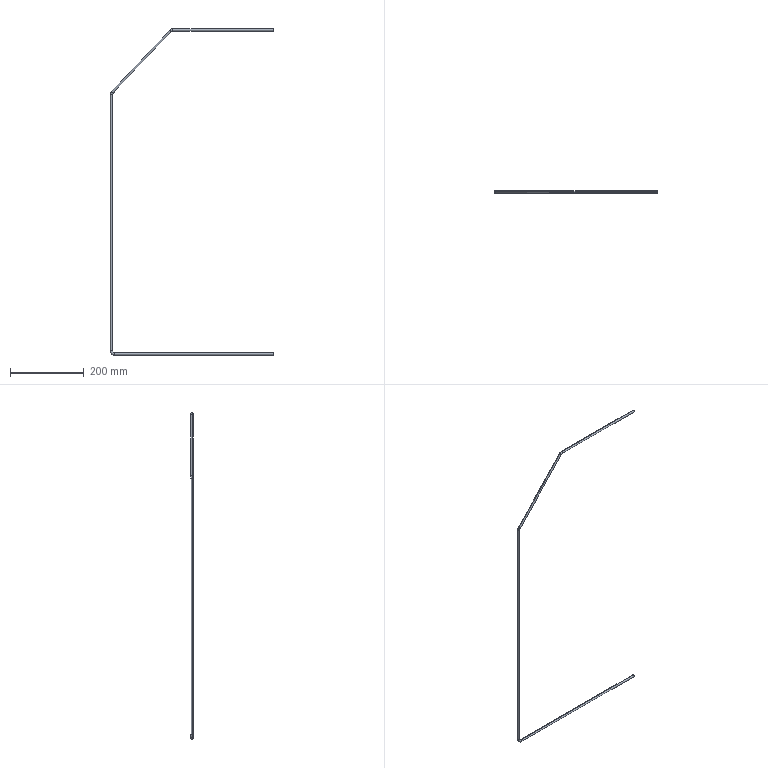Part | SolidWorks | features Sweep 1 | 1 solid | 16 faces | box 444.5 x 6 x 887 mm | volume 46970 mm3 | cylinder 8 | torus 6 | plane 2 | commonest cylinder face diameters 6 x8
STEP:
#1=CARTESIAN_POINT('',(-283.037,0.,880.262));
#2=VERTEX_POINT('',#1);
#3=CARTESIAN_POINT('',(-278.686,0.,876.131));
#4=VERTEX_POINT('',#3);
#5=CARTESIAN_POINT('',(-280.861,0.,878.197));
#6=DIRECTION('',(-0.6885,0.,-0.7252));
#7=DIRECTION('',(-0.7252,0.,0.6885));
#8=AXIS2_PLACEMENT_3D('',#5,#6,#7);
#9=CIRCLE('',#8,3.);
#10=EDGE_CURVE('',#2,#4,#9,.T.);
#11=ORIENTED_EDGE('',*,*,#10,.F.);
#12=CARTESIAN_POINT('',(-274.335,0.,884.));
#13=VERTEX_POINT('',#12);
#14=CARTESIAN_POINT('',(-274.335,0.,872.));
#15=DIRECTION('',(0.,1.,0.));
#16=DIRECTION('',(0.,0.,1.));
#17=AXIS2_PLACEMENT_3D('',#14,#15,#16);
#18=CIRCLE('',#17,12.);
#19=EDGE_CURVE('',#2,#13,#18,.T.);
#20=ORIENTED_EDGE('',*,*,#19,.T.);
#21=CARTESIAN_POINT('',(-274.335,0.,878.));
#22=VERTEX_POINT('',#21);
#23=CARTESIAN_POINT('',(-274.335,0.,881.));
#24=DIRECTION('',(-1.,0.,0.));
#25=DIRECTION('',(0.,0.,1.));
#26=AXIS2_PLACEMENT_3D('',#23,#24,#25);
#27=CIRCLE('',#26,3.);
#28=EDGE_CURVE('',#13,#22,#27,.T.);
#29=ORIENTED_EDGE('',*,*,#28,.T.);
#30=CARTESIAN_POINT('',(-274.335,0.,872.));
#31=DIRECTION('',(0.,1.,0.));
#32=DIRECTION('',(0.,0.,1.));
#33=AXIS2_PLACEMENT_3D('',#30,#31,#32);
#34=CIRCLE('',#33,6.);
#35=EDGE_CURVE('',#4,#22,#34,.T.);
#36=ORIENTED_EDGE('',*,*,#35,.F.);
#37=EDGE_LOOP('',(#11,#20,#29,#36));
#38=FACE_OUTER_BOUND('',#37,.T.);
#39=CARTESIAN_POINT('',(-274.335,0.,872.));
#40=DIRECTION('',(0.,1.,0.));
#41=DIRECTION('',(0.,0.,1.));
#42=AXIS2_PLACEMENT_3D('',#39,#40,#41);
#43=TOROIDAL_SURFACE('',#42,9.,3.);
#44=ADVANCED_FACE('',(#38),#43,.T.);
#45=CARTESIAN_POINT('',(-444.5,0.,705.408));
#46=VERTEX_POINT('',#45);
#47=CARTESIAN_POINT('',(-438.5,0.,705.408));
#48=VERTEX_POINT('',#47);
#49=CARTESIAN_POINT('',(-441.5,0.,705.408));
#50=DIRECTION('',(0.,0.,-1.));
#51=DIRECTION('',(-1.,0.,0.));
#52=AXIS2_PLACEMENT_3D('',#49,#50,#51);
#53=CIRCLE('',#52,3.);
#54=EDGE_CURVE('',#46,#48,#53,.T.);
#55=ORIENTED_EDGE('',*,*,#54,.F.);
#56=CARTESIAN_POINT('',(-441.203,0.,713.67));
#57=VERTEX_POINT('',#56);
#58=CARTESIAN_POINT('',(-432.5,0.,705.408));
#59=DIRECTION('',(0.,1.,0.));
#60=DIRECTION('',(0.,0.,1.));
#61=AXIS2_PLACEMENT_3D('',#58,#59,#60);
#62=CIRCLE('',#61,12.);
#63=EDGE_CURVE('',#46,#57,#62,.T.);
#64=ORIENTED_EDGE('',*,*,#63,.T.);
#65=CARTESIAN_POINT('',(-436.851,0.,709.539));
#66=VERTEX_POINT('',#65);
#67=CARTESIAN_POINT('',(-439.027,0.,711.605));
#68=DIRECTION('',(-0.6885,0.,-0.7252));
#69=DIRECTION('',(-0.7252,0.,0.6885));
#70=AXIS2_PLACEMENT_3D('',#67,#68,#69);
#71=CIRCLE('',#70,3.);
#72=EDGE_CURVE('',#57,#66,#71,.T.);
#73=ORIENTED_EDGE('',*,*,#72,.T.);
#74=CARTESIAN_POINT('',(-432.5,0.,705.408));
#75=DIRECTION('',(0.,1.,0.));
#76=DIRECTION('',(0.,0.,1.));
#77=AXIS2_PLACEMENT_3D('',#74,#75,#76);
#78=CIRCLE('',#77,6.);
#79=EDGE_CURVE('',#48,#66,#78,.T.);
#80=ORIENTED_EDGE('',*,*,#79,.F.);
#81=EDGE_LOOP('',(#55,#64,#73,#80));
#82=FACE_OUTER_BOUND('',#81,.T.);
#83=CARTESIAN_POINT('',(-432.5,0.,705.408));
#84=DIRECTION('',(0.,1.,0.));
#85=DIRECTION('',(0.,0.,1.));
#86=AXIS2_PLACEMENT_3D('',#83,#84,#85);
#87=TOROIDAL_SURFACE('',#86,9.,3.);
#88=ADVANCED_FACE('',(#82),#87,.T.);
#89=CARTESIAN_POINT('',(-432.5,0.,-3.));
#90=VERTEX_POINT('',#89);
#91=CARTESIAN_POINT('',(-432.5,0.,3.));
#92=VERTEX_POINT('',#91);
#93=CARTESIAN_POINT('',(-432.5,0.,0.));
#94=DIRECTION('',(1.,0.,0.));
#95=DIRECTION('',(0.,0.,-1.));
#96=AXIS2_PLACEMENT_3D('',#93,#94,#95);
#97=CIRCLE('',#96,3.);
#98=EDGE_CURVE('',#90,#92,#97,.T.);
#99=ORIENTED_EDGE('',*,*,#98,.F.);
#100=CARTESIAN_POINT('',(-444.5,0.,9.));
#101=VERTEX_POINT('',#100);
#102=CARTESIAN_POINT('',(-432.5,0.,9.));
#103=DIRECTION('',(0.,1.,0.));
#104=DIRECTION('',(0.,0.,1.));
#105=AXIS2_PLACEMENT_3D('',#102,#103,#104);
#106=CIRCLE('',#105,12.);
#107=EDGE_CURVE('',#90,#101,#106,.T.);
#108=ORIENTED_EDGE('',*,*,#107,.T.);
#109=CARTESIAN_POINT('',(-438.5,0.,9.));
#110=VERTEX_POINT('',#109);
#111=CARTESIAN_POINT('',(-441.5,0.,9.));
#112=DIRECTION('',(0.,0.,-1.));
#113=DIRECTION('',(-1.,0.,0.));
#114=AXIS2_PLACEMENT_3D('',#111,#112,#113);
#115=CIRCLE('',#114,3.);
#116=EDGE_CURVE('',#101,#110,#115,.T.);
#117=ORIENTED_EDGE('',*,*,#116,.T.);
#118=CARTESIAN_POINT('',(-432.5,0.,9.));
#119=DIRECTION('',(0.,1.,0.));
#120=DIRECTION('',(0.,0.,1.));
#121=AXIS2_PLACEMENT_3D('',#118,#119,#120);
#122=CIRCLE('',#121,6.);
#123=EDGE_CURVE('',#92,#110,#122,.T.);
#124=ORIENTED_EDGE('',*,*,#123,.F.);
#125=EDGE_LOOP('',(#99,#108,#117,#124));
#126=FACE_OUTER_BOUND('',#125,.T.);
#127=CARTESIAN_POINT('',(-432.5,0.,9.));
#128=DIRECTION('',(0.,1.,0.));
#129=DIRECTION('',(0.,0.,1.));
#130=AXIS2_PLACEMENT_3D('',#127,#128,#129);
#131=TOROIDAL_SURFACE('',#130,9.,3.);
#132=ADVANCED_FACE('',(#126),#131,.T.);
#133=ORIENTED_EDGE('',*,*,#28,.F.);
#134=CARTESIAN_POINT('',(0.,0.,884.));
#135=VERTEX_POINT('',#134);
#136=CARTESIAN_POINT('',(-274.335,0.,884.));
#137=DIRECTION('',(1.,0.,0.));
#138=VECTOR('',#137,1000.);
#139=LINE('',#136,#138);
#140=EDGE_CURVE('',#13,#135,#139,.T.);
#141=ORIENTED_EDGE('',*,*,#140,.T.);
#142=CARTESIAN_POINT('',(0.,0.,878.));
#143=VERTEX_POINT('',#142);
#144=CARTESIAN_POINT('',(0.,0.,881.));
#145=DIRECTION('',(-1.,0.,0.));
#146=DIRECTION('',(0.,0.,1.));
#147=AXIS2_PLACEMENT_3D('',#144,#145,#146);
#148=CIRCLE('',#147,3.);
#149=EDGE_CURVE('',#135,#143,#148,.T.);
#150=ORIENTED_EDGE('',*,*,#149,.T.);
#151=CARTESIAN_POINT('',(-274.335,0.,878.));
#152=DIRECTION('',(1.,0.,0.));
#153=VECTOR('',#152,1000.);
#154=LINE('',#151,#153);
#155=EDGE_CURVE('',#22,#143,#154,.T.);
#156=ORIENTED_EDGE('',*,*,#155,.F.);
#157=EDGE_LOOP('',(#133,#141,#150,#156));
#158=FACE_OUTER_BOUND('',#157,.T.);
#159=CARTESIAN_POINT('',(-274.335,0.,881.));
#160=DIRECTION('',(1.,0.,0.));
#161=DIRECTION('',(0.,0.,-1.));
#162=AXIS2_PLACEMENT_3D('',#159,#160,#161);
#163=CYLINDRICAL_SURFACE('',#162,3.);
#164=ADVANCED_FACE('',(#158),#163,.T.);
#165=ORIENTED_EDGE('',*,*,#72,.F.);
#166=CARTESIAN_POINT('',(-441.203,0.,713.67));
#167=DIRECTION('',(0.6885,0.,0.7252));
#168=VECTOR('',#167,1000.);
#169=LINE('',#166,#168);
#170=EDGE_CURVE('',#57,#2,#169,.T.);
#171=ORIENTED_EDGE('',*,*,#170,.T.);
#172=ORIENTED_EDGE('',*,*,#10,.T.);
#173=CARTESIAN_POINT('',(-436.851,0.,709.539));
#174=DIRECTION('',(0.6885,0.,0.7252));
#175=VECTOR('',#174,1000.);
#176=LINE('',#173,#175);
#177=EDGE_CURVE('',#66,#4,#176,.T.);
#178=ORIENTED_EDGE('',*,*,#177,.F.);
#179=EDGE_LOOP('',(#165,#171,#172,#178));
#180=FACE_OUTER_BOUND('',#179,.T.);
#181=CARTESIAN_POINT('',(-439.027,0.,711.605));
#182=DIRECTION('',(0.6885,0.,0.7252));
#183=DIRECTION('',(0.7252,0.,-0.6885));
#184=AXIS2_PLACEMENT_3D('',#181,#182,#183);
#185=CYLINDRICAL_SURFACE('',#184,3.);
#186=ADVANCED_FACE('',(#180),#185,.T.);
#187=ORIENTED_EDGE('',*,*,#116,.F.);
#188=CARTESIAN_POINT('',(-444.5,0.,9.));
#189=DIRECTION('',(0.,0.,1.));
#190=VECTOR('',#189,1000.);
#191=LINE('',#188,#190);
#192=EDGE_CURVE('',#101,#46,#191,.T.);
#193=ORIENTED_EDGE('',*,*,#192,.T.);
#194=ORIENTED_EDGE('',*,*,#54,.T.);
#195=CARTESIAN_POINT('',(-438.5,0.,9.));
#196=DIRECTION('',(0.,0.,1.));
#197=VECTOR('',#196,1000.);
#198=LINE('',#195,#197);
#199=EDGE_CURVE('',#110,#48,#198,.T.);
#200=ORIENTED_EDGE('',*,*,#199,.F.);
#201=EDGE_LOOP('',(#187,#193,#194,#200));
#202=FACE_OUTER_BOUND('',#201,.T.);
#203=CARTESIAN_POINT('',(-441.5,0.,9.));
#204=DIRECTION('',(0.,0.,1.));
#205=DIRECTION('',(1.,0.,0.));
#206=AXIS2_PLACEMENT_3D('',#203,#204,#205);
#207=CYLINDRICAL_SURFACE('',#206,3.);
#208=ADVANCED_FACE('',(#202),#207,.T.);
#209=CARTESIAN_POINT('',(0.,0.,-3.));
#210=VERTEX_POINT('',#209);
#211=CARTESIAN_POINT('',(0.,0.,3.));
#212=VERTEX_POINT('',#211);
#213=CARTESIAN_POINT('',(0.,0.,0.));
#214=DIRECTION('',(1.,0.,0.));
#215=DIRECTION('',(0.,0.,-1.));
#216=AXIS2_PLACEMENT_3D('',#213,#214,#215);
#217=CIRCLE('',#216,3.);
#218=EDGE_CURVE('',#210,#212,#217,.T.);
#219=ORIENTED_EDGE('',*,*,#218,.F.);
#220=CARTESIAN_POINT('',(0.,0.,-3.));
#221=DIRECTION('',(-1.,0.,0.));
#222=VECTOR('',#221,1000.);
#223=LINE('',#220,#222);
#224=EDGE_CURVE('',#210,#90,#223,.T.);
#225=ORIENTED_EDGE('',*,*,#224,.T.);
#226=ORIENTED_EDGE('',*,*,#98,.T.);
#227=CARTESIAN_POINT('',(0.,0.,3.));
#228=DIRECTION('',(-1.,0.,0.));
#229=VECTOR('',#228,1000.);
#230=LINE('',#227,#229);
#231=EDGE_CURVE('',#212,#92,#230,.T.);
#232=ORIENTED_EDGE('',*,*,#231,.F.);
#233=EDGE_LOOP('',(#219,#225,#226,#232));
#234=FACE_OUTER_BOUND('',#233,.T.);
#235=CARTESIAN_POINT('',(0.,0.,0.));
#236=DIRECTION('',(-1.,0.,0.));
#237=DIRECTION('',(0.,0.,1.));
#238=AXIS2_PLACEMENT_3D('',#235,#236,#237);
#239=CYLINDRICAL_SURFACE('',#238,3.);
#240=ADVANCED_FACE('',(#234),#239,.T.);
#241=ORIENTED_EDGE('',*,*,#140,.F.);
#242=CARTESIAN_POINT('',(-274.335,0.,881.));
#243=DIRECTION('',(-1.,0.,0.));
#244=DIRECTION('',(0.,0.,1.));
#245=AXIS2_PLACEMENT_3D('',#242,#243,#244);
#246=CIRCLE('',#245,3.);
#247=EDGE_CURVE('',#22,#13,#246,.T.);
#248=ORIENTED_EDGE('',*,*,#247,.F.);
#249=ORIENTED_EDGE('',*,*,#155,.T.);
#250=CARTESIAN_POINT('',(0.,0.,881.));
#251=DIRECTION('',(-1.,0.,0.));
#252=DIRECTION('',(0.,0.,1.));
#253=AXIS2_PLACEMENT_3D('',#250,#251,#252);
#254=CIRCLE('',#253,3.);
#255=EDGE_CURVE('',#143,#135,#254,.T.);
#256=ORIENTED_EDGE('',*,*,#255,.T.);
#257=EDGE_LOOP('',(#241,#248,#249,#256));
#258=FACE_OUTER_BOUND('',#257,.T.);
#259=CARTESIAN_POINT('',(-274.335,0.,881.));
#260=DIRECTION('',(1.,0.,0.));
#261=DIRECTION('',(0.,0.,-1.));
#262=AXIS2_PLACEMENT_3D('',#259,#260,#261);
#263=CYLINDRICAL_SURFACE('',#262,3.);
#264=ADVANCED_FACE('',(#258),#263,.T.);
#265=ORIENTED_EDGE('',*,*,#19,.F.);
#266=CARTESIAN_POINT('',(-280.861,0.,878.197));
#267=DIRECTION('',(-0.6885,0.,-0.7252));
#268=DIRECTION('',(-0.7252,0.,0.6885));
#269=AXIS2_PLACEMENT_3D('',#266,#267,#268);
#270=CIRCLE('',#269,3.);
#271=EDGE_CURVE('',#4,#2,#270,.T.);
#272=ORIENTED_EDGE('',*,*,#271,.F.);
#273=ORIENTED_EDGE('',*,*,#35,.T.);
#274=ORIENTED_EDGE('',*,*,#247,.T.);
#275=EDGE_LOOP('',(#265,#272,#273,#274));
#276=FACE_OUTER_BOUND('',#275,.T.);
#277=CARTESIAN_POINT('',(-274.335,0.,872.));
#278=DIRECTION('',(0.,1.,0.));
#279=DIRECTION('',(0.,0.,1.));
#280=AXIS2_PLACEMENT_3D('',#277,#278,#279);
#281=TOROIDAL_SURFACE('',#280,9.,3.);
#282=ADVANCED_FACE('',(#276),#281,.T.);
#283=ORIENTED_EDGE('',*,*,#170,.F.);
#284=CARTESIAN_POINT('',(-439.027,0.,711.605));
#285=DIRECTION('',(-0.6885,0.,-0.7252));
#286=DIRECTION('',(-0.7252,0.,0.6885));
#287=AXIS2_PLACEMENT_3D('',#284,#285,#286);
#288=CIRCLE('',#287,3.);
#289=EDGE_CURVE('',#66,#57,#288,.T.);
#290=ORIENTED_EDGE('',*,*,#289,.F.);
#291=ORIENTED_EDGE('',*,*,#177,.T.);
#292=ORIENTED_EDGE('',*,*,#271,.T.);
#293=EDGE_LOOP('',(#283,#290,#291,#292));
#294=FACE_OUTER_BOUND('',#293,.T.);
#295=CARTESIAN_POINT('',(-439.027,0.,711.605));
#296=DIRECTION('',(0.6885,0.,0.7252));
#297=DIRECTION('',(0.7252,0.,-0.6885));
#298=AXIS2_PLACEMENT_3D('',#295,#296,#297);
#299=CYLINDRICAL_SURFACE('',#298,3.);
#300=ADVANCED_FACE('',(#294),#299,.T.);
#301=ORIENTED_EDGE('',*,*,#63,.F.);
#302=CARTESIAN_POINT('',(-441.5,0.,705.408));
#303=DIRECTION('',(0.,0.,-1.));
#304=DIRECTION('',(-1.,0.,0.));
#305=AXIS2_PLACEMENT_3D('',#302,#303,#304);
#306=CIRCLE('',#305,3.);
#307=EDGE_CURVE('',#48,#46,#306,.T.);
#308=ORIENTED_EDGE('',*,*,#307,.F.);
#309=ORIENTED_EDGE('',*,*,#79,.T.);
#310=ORIENTED_EDGE('',*,*,#289,.T.);
#311=EDGE_LOOP('',(#301,#308,#309,#310));
#312=FACE_OUTER_BOUND('',#311,.T.);
#313=CARTESIAN_POINT('',(-432.5,0.,705.408));
#314=DIRECTION('',(0.,1.,0.));
#315=DIRECTION('',(0.,0.,1.));
#316=AXIS2_PLACEMENT_3D('',#313,#314,#315);
#317=TOROIDAL_SURFACE('',#316,9.,3.);
#318=ADVANCED_FACE('',(#312),#317,.T.);
#319=ORIENTED_EDGE('',*,*,#192,.F.);
#320=CARTESIAN_POINT('',(-441.5,0.,9.));
#321=DIRECTION('',(0.,0.,-1.));
#322=DIRECTION('',(-1.,0.,0.));
#323=AXIS2_PLACEMENT_3D('',#320,#321,#322);
#324=CIRCLE('',#323,3.);
#325=EDGE_CURVE('',#110,#101,#324,.T.);
#326=ORIENTED_EDGE('',*,*,#325,.F.);
#327=ORIENTED_EDGE('',*,*,#199,.T.);
#328=ORIENTED_EDGE('',*,*,#307,.T.);
#329=EDGE_LOOP('',(#319,#326,#327,#328));
#330=FACE_OUTER_BOUND('',#329,.T.);
#331=CARTESIAN_POINT('',(-441.5,0.,9.));
#332=DIRECTION('',(0.,0.,1.));
#333=DIRECTION('',(1.,0.,0.));
#334=AXIS2_PLACEMENT_3D('',#331,#332,#333);
#335=CYLINDRICAL_SURFACE('',#334,3.);
#336=ADVANCED_FACE('',(#330),#335,.T.);
#337=ORIENTED_EDGE('',*,*,#107,.F.);
#338=CARTESIAN_POINT('',(-432.5,0.,0.));
#339=DIRECTION('',(1.,0.,0.));
#340=DIRECTION('',(0.,0.,-1.));
#341=AXIS2_PLACEMENT_3D('',#338,#339,#340);
#342=CIRCLE('',#341,3.);
#343=EDGE_CURVE('',#92,#90,#342,.T.);
#344=ORIENTED_EDGE('',*,*,#343,.F.);
#345=ORIENTED_EDGE('',*,*,#123,.T.);
#346=ORIENTED_EDGE('',*,*,#325,.T.);
#347=EDGE_LOOP('',(#337,#344,#345,#346));
#348=FACE_OUTER_BOUND('',#347,.T.);
#349=CARTESIAN_POINT('',(-432.5,0.,9.));
#350=DIRECTION('',(0.,1.,0.));
#351=DIRECTION('',(0.,0.,1.));
#352=AXIS2_PLACEMENT_3D('',#349,#350,#351);
#353=TOROIDAL_SURFACE('',#352,9.,3.);
#354=ADVANCED_FACE('',(#348),#353,.T.);
#355=ORIENTED_EDGE('',*,*,#224,.F.);
#356=CARTESIAN_POINT('',(0.,0.,0.));
#357=DIRECTION('',(1.,0.,0.));
#358=DIRECTION('',(0.,0.,-1.));
#359=AXIS2_PLACEMENT_3D('',#356,#357,#358);
#360=CIRCLE('',#359,3.);
#361=EDGE_CURVE('',#212,#210,#360,.T.);
#362=ORIENTED_EDGE('',*,*,#361,.F.);
#363=ORIENTED_EDGE('',*,*,#231,.T.);
#364=ORIENTED_EDGE('',*,*,#343,.T.);
#365=EDGE_LOOP('',(#355,#362,#363,#364));
#366=FACE_OUTER_BOUND('',#365,.T.);
#367=CARTESIAN_POINT('',(0.,0.,0.));
#368=DIRECTION('',(-1.,0.,0.));
#369=DIRECTION('',(0.,0.,1.));
#370=AXIS2_PLACEMENT_3D('',#367,#368,#369);
#371=CYLINDRICAL_SURFACE('',#370,3.);
#372=ADVANCED_FACE('',(#366),#371,.T.);
#373=ORIENTED_EDGE('',*,*,#255,.F.);
#374=ORIENTED_EDGE('',*,*,#149,.F.);
#375=EDGE_LOOP('',(#373,#374));
#376=FACE_OUTER_BOUND('',#375,.T.);
#377=CARTESIAN_POINT('',(0.,0.,881.));
#378=DIRECTION('',(-1.,0.,0.));
#379=DIRECTION('',(0.,0.,1.));
#380=AXIS2_PLACEMENT_3D('',#377,#378,#379);
#381=PLANE('',#380);
#382=ADVANCED_FACE('',(#376),#381,.F.);
#383=ORIENTED_EDGE('',*,*,#361,.T.);
#384=ORIENTED_EDGE('',*,*,#218,.T.);
#385=EDGE_LOOP('',(#383,#384));
#386=FACE_OUTER_BOUND('',#385,.T.);
#387=CARTESIAN_POINT('',(0.,0.,0.));
#388=DIRECTION('',(1.,0.,0.));
#389=DIRECTION('',(0.,0.,-1.));
#390=AXIS2_PLACEMENT_3D('',#387,#388,#389);
#391=PLANE('',#390);
#392=ADVANCED_FACE('',(#386),#391,.T.);
#393=CLOSED_SHELL('',(#44,#88,#132,#164,#186,#208,#240,#264,#282,#300,#318,#336,#354,#372,#382,#392));
#394=MANIFOLD_SOLID_BREP('',#393);
#395=CARTESIAN_POINT('',(0.,0.,0.));
#396=DIRECTION('',(0.,0.,1.));
#397=DIRECTION('',(1.,0.,0.));
#398=AXIS2_PLACEMENT_3D('',#395,#396,#397);
#399=(LENGTH_UNIT()NAMED_UNIT(*)SI_UNIT(.MILLI.,.METRE.));
#400=UNCERTAINTY_MEASURE_WITH_UNIT(LENGTH_MEASURE(0.00001),#399,'','');
#401=(NAMED_UNIT(*)PLANE_ANGLE_UNIT()SI_UNIT($,.RADIAN.));
#402=(NAMED_UNIT(*)SI_UNIT($,.STERADIAN.)SOLID_ANGLE_UNIT());
#403=(GEOMETRIC_REPRESENTATION_CONTEXT(3)GLOBAL_UNCERTAINTY_ASSIGNED_CONTEXT((#400))GLOBAL_UNIT_ASSIGNED_CONTEXT((#399,#401,#402))REPRESENTATION_CONTEXT('',''));
#404=ADVANCED_BREP_SHAPE_REPRESENTATION('',(#394,#398),#403);